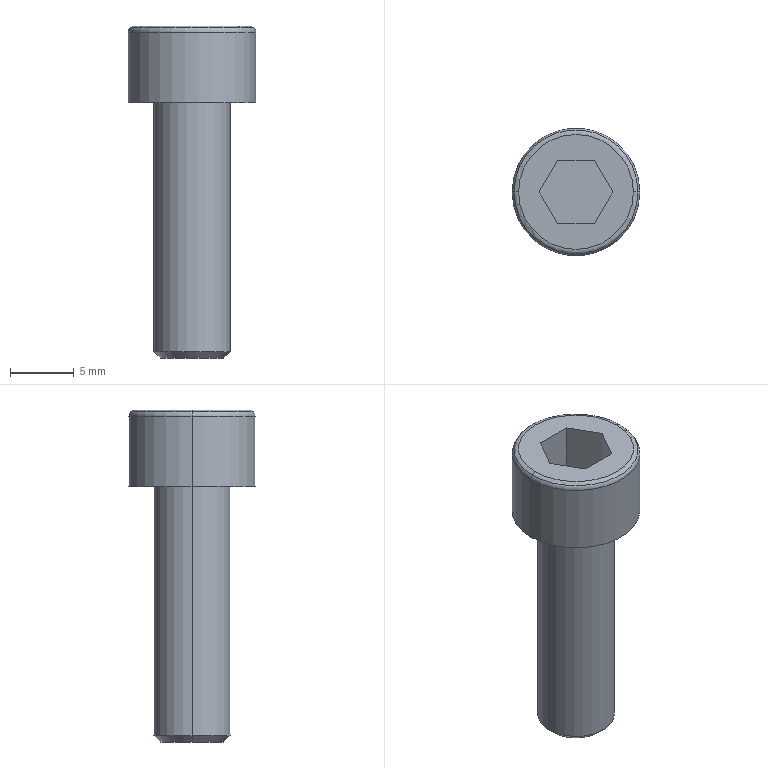Part | Creo | 1 solid | 20 faces | box 10 x 10 x 26 mm | volume 947.116 mm3 | plane 10 | cylinder 4 | torus 4 | cone 2 | commonest cylinder face diameters 6 x2 10 x2
STEP:
#1=CARTESIAN_POINT('',(-3.,-245.,-57.));
#2=VERTEX_POINT('',#1);
#3=CARTESIAN_POINT('',(3.,-245.,-57.));
#4=VERTEX_POINT('',#3);
#5=CARTESIAN_POINT('',(0.,-245.,-57.));
#6=DIRECTION('',(0.,0.,-1.));
#7=DIRECTION('',(-1.,0.,0.));
#8=AXIS2_PLACEMENT_3D('',#5,#6,#7);
#9=CIRCLE('',#8,3.);
#10=EDGE_CURVE('',#2,#4,#9,.T.);
#11=ORIENTED_EDGE('',*,*,#10,.T.);
#12=CARTESIAN_POINT('',(3.,-245.,-37.5));
#13=VERTEX_POINT('',#12);
#14=CARTESIAN_POINT('',(3.,-245.,-57.));
#15=DIRECTION('',(0.,0.,1.));
#16=VECTOR('',#15,19.5);
#17=LINE('',#14,#16);
#18=EDGE_CURVE('',#4,#13,#17,.T.);
#19=ORIENTED_EDGE('',*,*,#18,.T.);
#20=CARTESIAN_POINT('',(-3.,-245.,-37.5));
#21=VERTEX_POINT('',#20);
#22=CARTESIAN_POINT('',(0.,-245.,-37.5));
#23=DIRECTION('',(0.,0.,1.));
#24=DIRECTION('',(1.,0.,0.));
#25=AXIS2_PLACEMENT_3D('',#22,#23,#24);
#26=CIRCLE('',#25,3.);
#27=EDGE_CURVE('',#13,#21,#26,.T.);
#28=ORIENTED_EDGE('',*,*,#27,.T.);
#29=CARTESIAN_POINT('',(-3.,-245.,-57.));
#30=DIRECTION('',(0.,0.,1.));
#31=VECTOR('',#30,19.5);
#32=LINE('',#29,#31);
#33=EDGE_CURVE('',#2,#21,#32,.T.);
#34=ORIENTED_EDGE('',*,*,#33,.F.);
#35=EDGE_LOOP('',(#11,#19,#28,#34));
#36=FACE_OUTER_BOUND('',#35,.F.);
#37=CARTESIAN_POINT('',(0.,-245.,-57.5));
#38=DIRECTION('',(0.,0.,1.));
#39=DIRECTION('',(1.,0.,0.));
#40=AXIS2_PLACEMENT_3D('',#37,#38,#39);
#41=CYLINDRICAL_SURFACE('',#40,3.);
#42=ADVANCED_FACE('',(#36),#41,.T.);
#43=CARTESIAN_POINT('',(-2.5,-245.,-57.5));
#44=VERTEX_POINT('',#43);
#45=CARTESIAN_POINT('',(2.5,-245.,-57.5));
#46=VERTEX_POINT('',#45);
#47=CARTESIAN_POINT('',(0.,-245.,-57.5));
#48=DIRECTION('',(0.,0.,-1.));
#49=DIRECTION('',(-1.,0.,0.));
#50=AXIS2_PLACEMENT_3D('',#47,#48,#49);
#51=CIRCLE('',#50,2.5);
#52=EDGE_CURVE('',#44,#46,#51,.T.);
#53=ORIENTED_EDGE('',*,*,#52,.T.);
#54=CARTESIAN_POINT('',(2.5,-245.,-57.5));
#55=DIRECTION('',(0.7071,0.,0.7071));
#56=VECTOR('',#55,0.7071);
#57=LINE('',#54,#56);
#58=EDGE_CURVE('',#46,#4,#57,.T.);
#59=ORIENTED_EDGE('',*,*,#58,.T.);
#60=ORIENTED_EDGE('',*,*,#10,.F.);
#61=CARTESIAN_POINT('',(-2.5,-245.,-57.5));
#62=DIRECTION('',(-0.7071,0.,0.7071));
#63=VECTOR('',#62,0.7071);
#64=LINE('',#61,#63);
#65=EDGE_CURVE('',#44,#2,#64,.T.);
#66=ORIENTED_EDGE('',*,*,#65,.F.);
#67=EDGE_LOOP('',(#53,#59,#60,#66));
#68=FACE_OUTER_BOUND('',#67,.F.);
#69=CARTESIAN_POINT('',(0.,-245.,-57.25));
#70=DIRECTION('',(0.,0.,1.));
#71=DIRECTION('',(1.,0.,0.));
#72=AXIS2_PLACEMENT_3D('',#69,#70,#71);
#73=CONICAL_SURFACE('',#72,2.75,45.);
#74=ADVANCED_FACE('',(#68),#73,.T.);
#75=CARTESIAN_POINT('',(0.,-245.,-57.5));
#76=DIRECTION('',(0.,0.,-1.));
#77=DIRECTION('',(1.,0.,0.));
#78=AXIS2_PLACEMENT_3D('',#75,#76,#77);
#79=CIRCLE('',#78,2.5);
#80=EDGE_CURVE('',#46,#44,#79,.T.);
#81=ORIENTED_EDGE('',*,*,#80,.F.);
#82=ORIENTED_EDGE('',*,*,#52,.F.);
#83=EDGE_LOOP('',(#81,#82));
#84=FACE_OUTER_BOUND('',#83,.F.);
#85=CARTESIAN_POINT('',(0.,-245.,-57.5));
#86=DIRECTION('',(0.,0.,1.));
#87=DIRECTION('',(1.,0.,0.));
#88=AXIS2_PLACEMENT_3D('',#85,#86,#87);
#89=PLANE('',#88);
#90=ADVANCED_FACE('',(#84),#89,.F.);
#91=ORIENTED_EDGE('',*,*,#80,.T.);
#92=ORIENTED_EDGE('',*,*,#65,.T.);
#93=CARTESIAN_POINT('',(0.,-245.,-57.));
#94=DIRECTION('',(0.,0.,-1.));
#95=DIRECTION('',(1.,0.,0.));
#96=AXIS2_PLACEMENT_3D('',#93,#94,#95);
#97=CIRCLE('',#96,3.);
#98=EDGE_CURVE('',#4,#2,#97,.T.);
#99=ORIENTED_EDGE('',*,*,#98,.F.);
#100=ORIENTED_EDGE('',*,*,#58,.F.);
#101=EDGE_LOOP('',(#91,#92,#99,#100));
#102=FACE_OUTER_BOUND('',#101,.F.);
#103=CARTESIAN_POINT('',(0.,-245.,-57.25));
#104=DIRECTION('',(0.,0.,1.));
#105=DIRECTION('',(1.,0.,0.));
#106=AXIS2_PLACEMENT_3D('',#103,#104,#105);
#107=CONICAL_SURFACE('',#106,2.75,45.);
#108=ADVANCED_FACE('',(#102),#107,.T.);
#109=ORIENTED_EDGE('',*,*,#98,.T.);
#110=ORIENTED_EDGE('',*,*,#33,.T.);
#111=CARTESIAN_POINT('',(0.,-245.,-37.5));
#112=DIRECTION('',(0.,0.,1.));
#113=DIRECTION('',(-1.,0.,0.));
#114=AXIS2_PLACEMENT_3D('',#111,#112,#113);
#115=CIRCLE('',#114,3.);
#116=EDGE_CURVE('',#21,#13,#115,.T.);
#117=ORIENTED_EDGE('',*,*,#116,.T.);
#118=ORIENTED_EDGE('',*,*,#18,.F.);
#119=EDGE_LOOP('',(#109,#110,#117,#118));
#120=FACE_OUTER_BOUND('',#119,.F.);
#121=CARTESIAN_POINT('',(0.,-245.,-57.5));
#122=DIRECTION('',(0.,0.,1.));
#123=DIRECTION('',(1.,0.,0.));
#124=AXIS2_PLACEMENT_3D('',#121,#122,#123);
#125=CYLINDRICAL_SURFACE('',#124,3.);
#126=ADVANCED_FACE('',(#120),#125,.T.);
#127=CARTESIAN_POINT('',(5.,-245.,-37.5));
#128=VERTEX_POINT('',#127);
#129=CARTESIAN_POINT('',(-5.,-245.,-37.5));
#130=VERTEX_POINT('',#129);
#131=CARTESIAN_POINT('',(0.,-245.,-37.5));
#132=DIRECTION('',(0.,0.,-1.));
#133=DIRECTION('',(1.,0.,0.));
#134=AXIS2_PLACEMENT_3D('',#131,#132,#133);
#135=CIRCLE('',#134,5.);
#136=EDGE_CURVE('',#128,#130,#135,.T.);
#137=ORIENTED_EDGE('',*,*,#136,.F.);
#138=CARTESIAN_POINT('',(0.,-245.,-37.5));
#139=DIRECTION('',(0.,0.,-1.));
#140=DIRECTION('',(-1.,0.,0.));
#141=AXIS2_PLACEMENT_3D('',#138,#139,#140);
#142=CIRCLE('',#141,5.);
#143=EDGE_CURVE('',#130,#128,#142,.T.);
#144=ORIENTED_EDGE('',*,*,#143,.F.);
#145=EDGE_LOOP('',(#137,#144));
#146=FACE_OUTER_BOUND('',#145,.F.);
#147=ORIENTED_EDGE('',*,*,#27,.F.);
#148=ORIENTED_EDGE('',*,*,#116,.F.);
#149=EDGE_LOOP('',(#147,#148));
#150=FACE_BOUND('',#149,.F.);
#151=CARTESIAN_POINT('',(0.,-245.,-37.5));
#152=DIRECTION('',(0.,0.,-1.));
#153=DIRECTION('',(-1.,0.,0.));
#154=AXIS2_PLACEMENT_3D('',#151,#152,#153);
#155=PLANE('',#154);
#156=ADVANCED_FACE('',(#146,#150),#155,.T.);
#157=CARTESIAN_POINT('',(-5.,-245.,-32.));
#158=VERTEX_POINT('',#157);
#159=CARTESIAN_POINT('',(5.,-245.,-32.));
#160=VERTEX_POINT('',#159);
#161=CARTESIAN_POINT('',(0.,-245.,-32.));
#162=DIRECTION('',(0.,0.,1.));
#163=DIRECTION('',(-1.,0.,0.));
#164=AXIS2_PLACEMENT_3D('',#161,#162,#163);
#165=CIRCLE('',#164,5.);
#166=EDGE_CURVE('',#158,#160,#165,.T.);
#167=ORIENTED_EDGE('',*,*,#166,.T.);
#168=CARTESIAN_POINT('',(5.,-245.,-37.5));
#169=DIRECTION('',(0.,0.,1.));
#170=VECTOR('',#169,5.5);
#171=LINE('',#168,#170);
#172=EDGE_CURVE('',#128,#160,#171,.T.);
#173=ORIENTED_EDGE('',*,*,#172,.F.);
#174=ORIENTED_EDGE('',*,*,#136,.T.);
#175=CARTESIAN_POINT('',(-5.,-245.,-37.5));
#176=DIRECTION('',(0.,0.,1.));
#177=VECTOR('',#176,5.5);
#178=LINE('',#175,#177);
#179=EDGE_CURVE('',#130,#158,#178,.T.);
#180=ORIENTED_EDGE('',*,*,#179,.T.);
#181=EDGE_LOOP('',(#167,#173,#174,#180));
#182=FACE_OUTER_BOUND('',#181,.F.);
#183=CARTESIAN_POINT('',(0.,-245.,-37.5));
#184=DIRECTION('',(0.,0.,1.));
#185=DIRECTION('',(1.,0.,0.));
#186=AXIS2_PLACEMENT_3D('',#183,#184,#185);
#187=CYLINDRICAL_SURFACE('',#186,5.);
#188=ADVANCED_FACE('',(#182),#187,.T.);
#189=ORIENTED_EDGE('',*,*,#166,.F.);
#190=CARTESIAN_POINT('',(-4.854,-245.,-31.646));
#191=VERTEX_POINT('',#190);
#192=CARTESIAN_POINT('',(-4.5,-245.,-32.));
#193=DIRECTION('',(0.,1.,0.));
#194=DIRECTION('',(-1.,0.,0.));
#195=AXIS2_PLACEMENT_3D('',#192,#193,#194);
#196=CIRCLE('',#195,0.5);
#197=EDGE_CURVE('',#158,#191,#196,.T.);
#198=ORIENTED_EDGE('',*,*,#197,.T.);
#199=CARTESIAN_POINT('',(4.854,-245.,-31.646));
#200=VERTEX_POINT('',#199);
#201=CARTESIAN_POINT('',(0.,-245.,-31.646));
#202=DIRECTION('',(0.,0.,1.));
#203=DIRECTION('',(-1.,0.,0.));
#204=AXIS2_PLACEMENT_3D('',#201,#202,#203);
#205=CIRCLE('',#204,4.854);
#206=EDGE_CURVE('',#191,#200,#205,.T.);
#207=ORIENTED_EDGE('',*,*,#206,.T.);
#208=CARTESIAN_POINT('',(4.5,-245.,-32.));
#209=DIRECTION('',(0.,-1.,0.));
#210=DIRECTION('',(1.,0.,0.));
#211=AXIS2_PLACEMENT_3D('',#208,#209,#210);
#212=CIRCLE('',#211,0.5);
#213=EDGE_CURVE('',#160,#200,#212,.T.);
#214=ORIENTED_EDGE('',*,*,#213,.F.);
#215=EDGE_LOOP('',(#189,#198,#207,#214));
#216=FACE_OUTER_BOUND('',#215,.F.);
#217=CARTESIAN_POINT('',(0.,-245.,-32.));
#218=DIRECTION('',(0.,0.,1.));
#219=DIRECTION('',(1.,0.,0.));
#220=AXIS2_PLACEMENT_3D('',#217,#218,#219);
#221=TOROIDAL_SURFACE('',#220,4.5,0.5);
#222=ADVANCED_FACE('',(#216),#221,.T.);
#223=CARTESIAN_POINT('',(0.,-245.,-32.));
#224=DIRECTION('',(0.,0.,1.));
#225=DIRECTION('',(1.,0.,0.));
#226=AXIS2_PLACEMENT_3D('',#223,#224,#225);
#227=CIRCLE('',#226,5.);
#228=EDGE_CURVE('',#160,#158,#227,.T.);
#229=ORIENTED_EDGE('',*,*,#228,.F.);
#230=ORIENTED_EDGE('',*,*,#213,.T.);
#231=CARTESIAN_POINT('',(0.,-245.,-31.646));
#232=DIRECTION('',(0.,0.,1.));
#233=DIRECTION('',(1.,0.,0.));
#234=AXIS2_PLACEMENT_3D('',#231,#232,#233);
#235=CIRCLE('',#234,4.854);
#236=EDGE_CURVE('',#200,#191,#235,.T.);
#237=ORIENTED_EDGE('',*,*,#236,.T.);
#238=ORIENTED_EDGE('',*,*,#197,.F.);
#239=EDGE_LOOP('',(#229,#230,#237,#238));
#240=FACE_OUTER_BOUND('',#239,.F.);
#241=CARTESIAN_POINT('',(0.,-245.,-32.));
#242=DIRECTION('',(0.,0.,1.));
#243=DIRECTION('',(1.,0.,0.));
#244=AXIS2_PLACEMENT_3D('',#241,#242,#243);
#245=TOROIDAL_SURFACE('',#244,4.5,0.5);
#246=ADVANCED_FACE('',(#240),#245,.T.);
#247=ORIENTED_EDGE('',*,*,#228,.T.);
#248=ORIENTED_EDGE('',*,*,#179,.F.);
#249=ORIENTED_EDGE('',*,*,#143,.T.);
#250=ORIENTED_EDGE('',*,*,#172,.T.);
#251=EDGE_LOOP('',(#247,#248,#249,#250));
#252=FACE_OUTER_BOUND('',#251,.F.);
#253=CARTESIAN_POINT('',(0.,-245.,-37.5));
#254=DIRECTION('',(0.,0.,1.));
#255=DIRECTION('',(1.,0.,0.));
#256=AXIS2_PLACEMENT_3D('',#253,#254,#255);
#257=CYLINDRICAL_SURFACE('',#256,5.);
#258=ADVANCED_FACE('',(#252),#257,.T.);
#259=CARTESIAN_POINT('',(4.5,-245.,-31.5));
#260=VERTEX_POINT('',#259);
#261=CARTESIAN_POINT('',(-4.5,-245.,-31.5));
#262=VERTEX_POINT('',#261);
#263=CARTESIAN_POINT('',(0.,-245.,-31.5));
#264=DIRECTION('',(0.,0.,1.));
#265=DIRECTION('',(1.,0.,0.));
#266=AXIS2_PLACEMENT_3D('',#263,#264,#265);
#267=CIRCLE('',#266,4.5);
#268=EDGE_CURVE('',#260,#262,#267,.T.);
#269=ORIENTED_EDGE('',*,*,#268,.T.);
#270=CARTESIAN_POINT('',(-4.5,-245.,-32.));
#271=DIRECTION('',(0.,1.,0.));
#272=DIRECTION('',(-0.7071,0.,0.7071));
#273=AXIS2_PLACEMENT_3D('',#270,#271,#272);
#274=CIRCLE('',#273,0.5);
#275=EDGE_CURVE('',#191,#262,#274,.T.);
#276=ORIENTED_EDGE('',*,*,#275,.F.);
#277=ORIENTED_EDGE('',*,*,#236,.F.);
#278=CARTESIAN_POINT('',(4.5,-245.,-32.));
#279=DIRECTION('',(0.,-1.,0.));
#280=DIRECTION('',(0.7071,0.,0.7071));
#281=AXIS2_PLACEMENT_3D('',#278,#279,#280);
#282=CIRCLE('',#281,0.5);
#283=EDGE_CURVE('',#200,#260,#282,.T.);
#284=ORIENTED_EDGE('',*,*,#283,.T.);
#285=EDGE_LOOP('',(#269,#276,#277,#284));
#286=FACE_OUTER_BOUND('',#285,.F.);
#287=CARTESIAN_POINT('',(0.,-245.,-32.));
#288=DIRECTION('',(0.,0.,1.));
#289=DIRECTION('',(1.,0.,0.));
#290=AXIS2_PLACEMENT_3D('',#287,#288,#289);
#291=TOROIDAL_SURFACE('',#290,4.5,0.5);
#292=ADVANCED_FACE('',(#286),#291,.T.);
#293=ORIENTED_EDGE('',*,*,#268,.F.);
#294=CARTESIAN_POINT('',(0.,-245.,-31.5));
#295=DIRECTION('',(0.,0.,1.));
#296=DIRECTION('',(-1.,0.,0.));
#297=AXIS2_PLACEMENT_3D('',#294,#295,#296);
#298=CIRCLE('',#297,4.5);
#299=EDGE_CURVE('',#262,#260,#298,.T.);
#300=ORIENTED_EDGE('',*,*,#299,.F.);
#301=EDGE_LOOP('',(#293,#300));
#302=FACE_OUTER_BOUND('',#301,.F.);
#303=CARTESIAN_POINT('',(1.443,-247.5,-31.5));
#304=VERTEX_POINT('',#303);
#305=CARTESIAN_POINT('',(-1.443,-247.5,-31.5));
#306=VERTEX_POINT('',#305);
#307=CARTESIAN_POINT('',(1.443,-247.5,-31.5));
#308=DIRECTION('',(-1.,0.,0.));
#309=VECTOR('',#308,2.887);
#310=LINE('',#307,#309);
#311=EDGE_CURVE('',#304,#306,#310,.T.);
#312=ORIENTED_EDGE('',*,*,#311,.F.);
#313=CARTESIAN_POINT('',(2.887,-245.,-31.5));
#314=VERTEX_POINT('',#313);
#315=CARTESIAN_POINT('',(2.887,-245.,-31.5));
#316=DIRECTION('',(-0.5,-0.866,0.));
#317=VECTOR('',#316,2.887);
#318=LINE('',#315,#317);
#319=EDGE_CURVE('',#314,#304,#318,.T.);
#320=ORIENTED_EDGE('',*,*,#319,.F.);
#321=CARTESIAN_POINT('',(1.443,-242.5,-31.5));
#322=VERTEX_POINT('',#321);
#323=CARTESIAN_POINT('',(1.443,-242.5,-31.5));
#324=DIRECTION('',(0.5,-0.866,0.));
#325=VECTOR('',#324,2.887);
#326=LINE('',#323,#325);
#327=EDGE_CURVE('',#322,#314,#326,.T.);
#328=ORIENTED_EDGE('',*,*,#327,.F.);
#329=CARTESIAN_POINT('',(-1.443,-242.5,-31.5));
#330=VERTEX_POINT('',#329);
#331=CARTESIAN_POINT('',(-1.443,-242.5,-31.5));
#332=DIRECTION('',(1.,0.,0.));
#333=VECTOR('',#332,2.887);
#334=LINE('',#331,#333);
#335=EDGE_CURVE('',#330,#322,#334,.T.);
#336=ORIENTED_EDGE('',*,*,#335,.F.);
#337=CARTESIAN_POINT('',(-2.887,-245.,-31.5));
#338=VERTEX_POINT('',#337);
#339=CARTESIAN_POINT('',(-2.887,-245.,-31.5));
#340=DIRECTION('',(0.5,0.866,0.));
#341=VECTOR('',#340,2.887);
#342=LINE('',#339,#341);
#343=EDGE_CURVE('',#338,#330,#342,.T.);
#344=ORIENTED_EDGE('',*,*,#343,.F.);
#345=CARTESIAN_POINT('',(-1.443,-247.5,-31.5));
#346=DIRECTION('',(-0.5,0.866,0.));
#347=VECTOR('',#346,2.887);
#348=LINE('',#345,#347);
#349=EDGE_CURVE('',#306,#338,#348,.T.);
#350=ORIENTED_EDGE('',*,*,#349,.F.);
#351=EDGE_LOOP('',(#312,#320,#328,#336,#344,#350));
#352=FACE_BOUND('',#351,.F.);
#353=CARTESIAN_POINT('',(0.,-245.,-31.5));
#354=DIRECTION('',(0.,0.,1.));
#355=DIRECTION('',(1.,0.,0.));
#356=AXIS2_PLACEMENT_3D('',#353,#354,#355);
#357=PLANE('',#356);
#358=ADVANCED_FACE('',(#302,#352),#357,.T.);
#359=ORIENTED_EDGE('',*,*,#299,.T.);
#360=ORIENTED_EDGE('',*,*,#283,.F.);
#361=ORIENTED_EDGE('',*,*,#206,.F.);
#362=ORIENTED_EDGE('',*,*,#275,.T.);
#363=EDGE_LOOP('',(#359,#360,#361,#362));
#364=FACE_OUTER_BOUND('',#363,.F.);
#365=CARTESIAN_POINT('',(0.,-245.,-32.));
#366=DIRECTION('',(0.,0.,1.));
#367=DIRECTION('',(1.,0.,0.));
#368=AXIS2_PLACEMENT_3D('',#365,#366,#367);
#369=TOROIDAL_SURFACE('',#368,4.5,0.5);
#370=ADVANCED_FACE('',(#364),#369,.T.);
#371=ORIENTED_EDGE('',*,*,#311,.T.);
#372=CARTESIAN_POINT('',(-1.443,-247.5,-35.46));
#373=VERTEX_POINT('',#372);
#374=CARTESIAN_POINT('',(-1.443,-247.5,-31.5));
#375=DIRECTION('',(0.,0.,-1.));
#376=VECTOR('',#375,3.96);
#377=LINE('',#374,#376);
#378=EDGE_CURVE('',#306,#373,#377,.T.);
#379=ORIENTED_EDGE('',*,*,#378,.T.);
#380=CARTESIAN_POINT('',(1.443,-247.5,-35.46));
#381=VERTEX_POINT('',#380);
#382=CARTESIAN_POINT('',(1.443,-247.5,-35.46));
#383=DIRECTION('',(-1.,0.,0.));
#384=VECTOR('',#383,2.887);
#385=LINE('',#382,#384);
#386=EDGE_CURVE('',#381,#373,#385,.T.);
#387=ORIENTED_EDGE('',*,*,#386,.F.);
#388=CARTESIAN_POINT('',(1.443,-247.5,-31.5));
#389=DIRECTION('',(0.,0.,-1.));
#390=VECTOR('',#389,3.96);
#391=LINE('',#388,#390);
#392=EDGE_CURVE('',#304,#381,#391,.T.);
#393=ORIENTED_EDGE('',*,*,#392,.F.);
#394=EDGE_LOOP('',(#371,#379,#387,#393));
#395=FACE_OUTER_BOUND('',#394,.F.);
#396=CARTESIAN_POINT('',(-1.443,-247.5,-35.46));
#397=DIRECTION('',(0.,-1.,0.));
#398=DIRECTION('',(0.,0.,-1.));
#399=AXIS2_PLACEMENT_3D('',#396,#397,#398);
#400=PLANE('',#399);
#401=ADVANCED_FACE('',(#395),#400,.F.);
#402=ORIENTED_EDGE('',*,*,#349,.T.);
#403=CARTESIAN_POINT('',(-2.887,-245.,-35.46));
#404=VERTEX_POINT('',#403);
#405=CARTESIAN_POINT('',(-2.887,-245.,-31.5));
#406=DIRECTION('',(0.,0.,-1.));
#407=VECTOR('',#406,3.96);
#408=LINE('',#405,#407);
#409=EDGE_CURVE('',#338,#404,#408,.T.);
#410=ORIENTED_EDGE('',*,*,#409,.T.);
#411=CARTESIAN_POINT('',(-2.887,-245.,-35.46));
#412=DIRECTION('',(0.5,-0.866,0.));
#413=VECTOR('',#412,2.887);
#414=LINE('',#411,#413);
#415=EDGE_CURVE('',#404,#373,#414,.T.);
#416=ORIENTED_EDGE('',*,*,#415,.T.);
#417=ORIENTED_EDGE('',*,*,#378,.F.);
#418=EDGE_LOOP('',(#402,#410,#416,#417));
#419=FACE_OUTER_BOUND('',#418,.F.);
#420=CARTESIAN_POINT('',(-2.887,-245.,-35.46));
#421=DIRECTION('',(-0.866,-0.5,0.));
#422=DIRECTION('',(0.5,-0.866,0.));
#423=AXIS2_PLACEMENT_3D('',#420,#421,#422);
#424=PLANE('',#423);
#425=ADVANCED_FACE('',(#419),#424,.F.);
#426=ORIENTED_EDGE('',*,*,#343,.T.);
#427=CARTESIAN_POINT('',(-1.443,-242.5,-35.46));
#428=VERTEX_POINT('',#427);
#429=CARTESIAN_POINT('',(-1.443,-242.5,-31.5));
#430=DIRECTION('',(0.,0.,-1.));
#431=VECTOR('',#430,3.96);
#432=LINE('',#429,#431);
#433=EDGE_CURVE('',#330,#428,#432,.T.);
#434=ORIENTED_EDGE('',*,*,#433,.T.);
#435=CARTESIAN_POINT('',(-1.443,-242.5,-35.46));
#436=DIRECTION('',(-0.5,-0.866,0.));
#437=VECTOR('',#436,2.887);
#438=LINE('',#435,#437);
#439=EDGE_CURVE('',#428,#404,#438,.T.);
#440=ORIENTED_EDGE('',*,*,#439,.T.);
#441=ORIENTED_EDGE('',*,*,#409,.F.);
#442=EDGE_LOOP('',(#426,#434,#440,#441));
#443=FACE_OUTER_BOUND('',#442,.F.);
#444=CARTESIAN_POINT('',(-1.443,-242.5,-35.46));
#445=DIRECTION('',(-0.866,0.5,0.));
#446=DIRECTION('',(-0.5,-0.866,0.));
#447=AXIS2_PLACEMENT_3D('',#444,#445,#446);
#448=PLANE('',#447);
#449=ADVANCED_FACE('',(#443),#448,.F.);
#450=ORIENTED_EDGE('',*,*,#335,.T.);
#451=CARTESIAN_POINT('',(1.443,-242.5,-35.46));
#452=VERTEX_POINT('',#451);
#453=CARTESIAN_POINT('',(1.443,-242.5,-31.5));
#454=DIRECTION('',(0.,0.,-1.));
#455=VECTOR('',#454,3.96);
#456=LINE('',#453,#455);
#457=EDGE_CURVE('',#322,#452,#456,.T.);
#458=ORIENTED_EDGE('',*,*,#457,.T.);
#459=CARTESIAN_POINT('',(-1.443,-242.5,-35.46));
#460=DIRECTION('',(1.,0.,0.));
#461=VECTOR('',#460,2.887);
#462=LINE('',#459,#461);
#463=EDGE_CURVE('',#428,#452,#462,.T.);
#464=ORIENTED_EDGE('',*,*,#463,.F.);
#465=ORIENTED_EDGE('',*,*,#433,.F.);
#466=EDGE_LOOP('',(#450,#458,#464,#465));
#467=FACE_OUTER_BOUND('',#466,.F.);
#468=CARTESIAN_POINT('',(1.443,-242.5,-35.46));
#469=DIRECTION('',(0.,1.,0.));
#470=DIRECTION('',(0.,0.,1.));
#471=AXIS2_PLACEMENT_3D('',#468,#469,#470);
#472=PLANE('',#471);
#473=ADVANCED_FACE('',(#467),#472,.F.);
#474=ORIENTED_EDGE('',*,*,#327,.T.);
#475=CARTESIAN_POINT('',(2.887,-245.,-35.46));
#476=VERTEX_POINT('',#475);
#477=CARTESIAN_POINT('',(2.887,-245.,-31.5));
#478=DIRECTION('',(0.,0.,-1.));
#479=VECTOR('',#478,3.96);
#480=LINE('',#477,#479);
#481=EDGE_CURVE('',#314,#476,#480,.T.);
#482=ORIENTED_EDGE('',*,*,#481,.T.);
#483=CARTESIAN_POINT('',(2.887,-245.,-35.46));
#484=DIRECTION('',(-0.5,0.866,0.));
#485=VECTOR('',#484,2.887);
#486=LINE('',#483,#485);
#487=EDGE_CURVE('',#476,#452,#486,.T.);
#488=ORIENTED_EDGE('',*,*,#487,.T.);
#489=ORIENTED_EDGE('',*,*,#457,.F.);
#490=EDGE_LOOP('',(#474,#482,#488,#489));
#491=FACE_OUTER_BOUND('',#490,.F.);
#492=CARTESIAN_POINT('',(2.887,-245.,-35.46));
#493=DIRECTION('',(0.866,0.5,0.));
#494=DIRECTION('',(-0.5,0.866,0.));
#495=AXIS2_PLACEMENT_3D('',#492,#493,#494);
#496=PLANE('',#495);
#497=ADVANCED_FACE('',(#491),#496,.F.);
#498=ORIENTED_EDGE('',*,*,#319,.T.);
#499=ORIENTED_EDGE('',*,*,#392,.T.);
#500=CARTESIAN_POINT('',(1.443,-247.5,-35.46));
#501=DIRECTION('',(0.5,0.866,0.));
#502=VECTOR('',#501,2.887);
#503=LINE('',#500,#502);
#504=EDGE_CURVE('',#381,#476,#503,.T.);
#505=ORIENTED_EDGE('',*,*,#504,.T.);
#506=ORIENTED_EDGE('',*,*,#481,.F.);
#507=EDGE_LOOP('',(#498,#499,#505,#506));
#508=FACE_OUTER_BOUND('',#507,.F.);
#509=CARTESIAN_POINT('',(1.443,-247.5,-35.46));
#510=DIRECTION('',(0.866,-0.5,0.));
#511=DIRECTION('',(0.5,0.866,0.));
#512=AXIS2_PLACEMENT_3D('',#509,#510,#511);
#513=PLANE('',#512);
#514=ADVANCED_FACE('',(#508),#513,.F.);
#515=ORIENTED_EDGE('',*,*,#386,.T.);
#516=ORIENTED_EDGE('',*,*,#415,.F.);
#517=ORIENTED_EDGE('',*,*,#439,.F.);
#518=ORIENTED_EDGE('',*,*,#463,.T.);
#519=ORIENTED_EDGE('',*,*,#487,.F.);
#520=ORIENTED_EDGE('',*,*,#504,.F.);
#521=EDGE_LOOP('',(#515,#516,#517,#518,#519,#520));
#522=FACE_OUTER_BOUND('',#521,.F.);
#523=CARTESIAN_POINT('',(1.443,-247.5,-35.46));
#524=DIRECTION('',(0.,0.,1.));
#525=DIRECTION('',(1.,0.,0.));
#526=AXIS2_PLACEMENT_3D('',#523,#524,#525);
#527=PLANE('',#526);
#528=ADVANCED_FACE('',(#522),#527,.T.);
#529=CLOSED_SHELL('',(#42,#74,#90,#108,#126,#156,#188,#222,#246,#258,#292,#358,#370,#401,#425,#449,#473,#497,#514,#528));
#530=MANIFOLD_SOLID_BREP('',#529);
#531=(LENGTH_UNIT()NAMED_UNIT(*)SI_UNIT(.MILLI.,.METRE.));
#532=UNCERTAINTY_MEASURE_WITH_UNIT(LENGTH_MEASURE(0.00296),#531,'','');
#533=(NAMED_UNIT(*)PLANE_ANGLE_UNIT()SI_UNIT($,.RADIAN.));
#534=PLANE_ANGLE_MEASURE_WITH_UNIT(PLANE_ANGLE_MEASURE(0.01745),#533);
#535=(CONVERSION_BASED_UNIT('DEGREE',#534)NAMED_UNIT(*)PLANE_ANGLE_UNIT());
#536=(NAMED_UNIT(*)SI_UNIT($,.STERADIAN.)SOLID_ANGLE_UNIT());
#537=(GEOMETRIC_REPRESENTATION_CONTEXT(3)GLOBAL_UNCERTAINTY_ASSIGNED_CONTEXT((#532))GLOBAL_UNIT_ASSIGNED_CONTEXT((#531,#535,#536))REPRESENTATION_CONTEXT('',''));
#538=ADVANCED_BREP_SHAPE_REPRESENTATION('',(#530),#537);